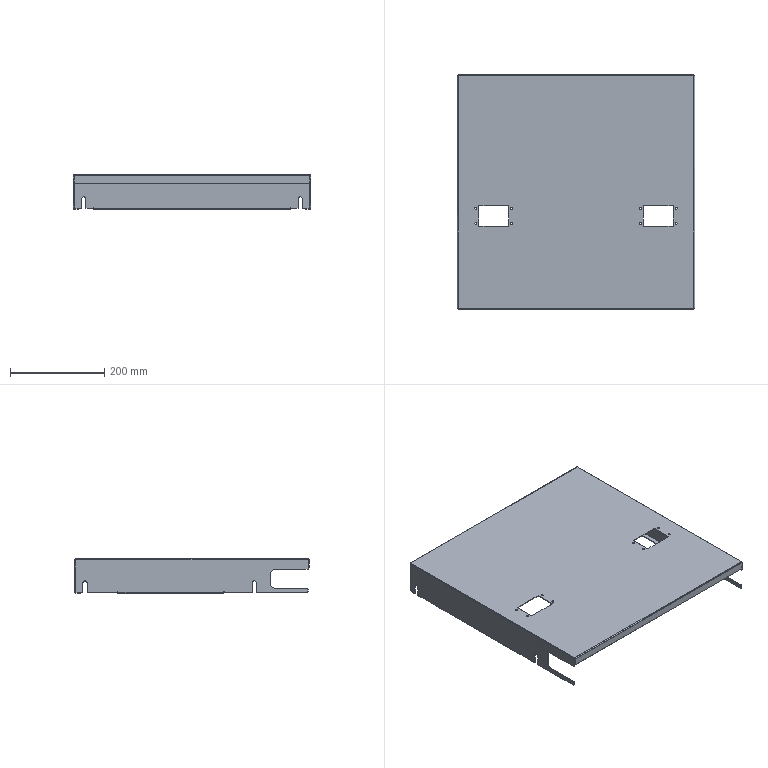Part | SolidWorks | features BaseBody 1 | 1 solid | 162 faces | box 505 x 498 x 73 mm | volume 537939 mm3 | plane 98 | cylinder 56 | spline 8 | commonest cylinder face diameters 4.5 x16 9 x12 6 x10 1.473 x7 4.473 x7 20 x4